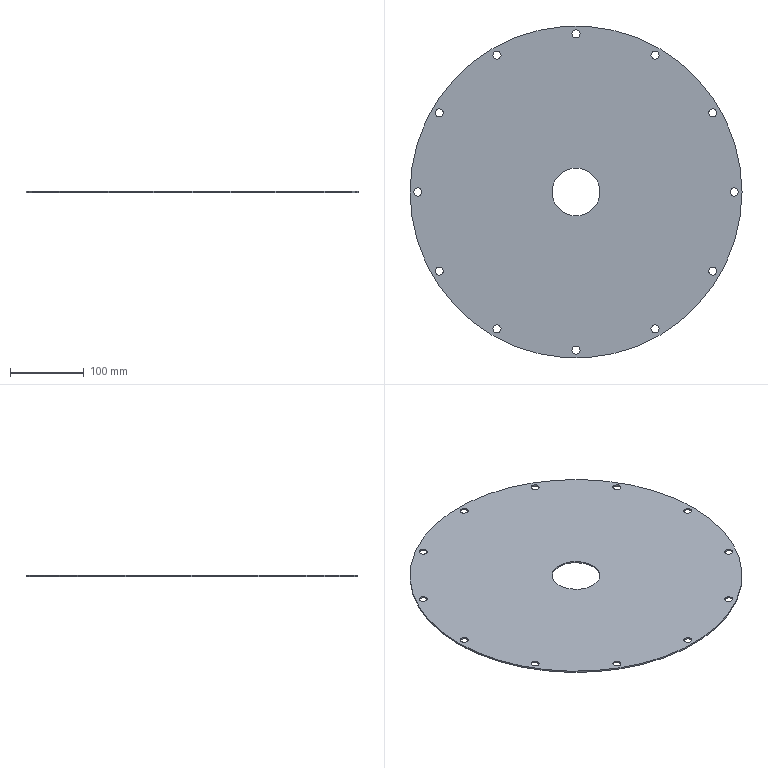Part | SolidWorks | features BaseBody 1 | 1 solid | 30 faces | box 450 x 450 x 2 mm | volume 309169 mm3 | cylinder 28 | plane 2 | commonest cylinder face diameters 11 x24 65 x2 450 x2
STEP:
#1=CARTESIAN_POINT('',(32.5,0.,2.));
#2=VERTEX_POINT('',#1);
#3=CARTESIAN_POINT('',(-32.5,0.,2.));
#4=VERTEX_POINT('',#3);
#5=CARTESIAN_POINT('',(0.,0.,2.));
#6=DIRECTION('',(0.,0.,-1.));
#7=DIRECTION('',(-1.,0.,0.));
#8=AXIS2_PLACEMENT_3D('',#5,#6,#7);
#9=CIRCLE('',#8,32.5);
#10=EDGE_CURVE('',#2,#4,#9,.T.);
#11=ORIENTED_EDGE('',*,*,#10,.F.);
#12=CARTESIAN_POINT('',(32.5,0.,0.));
#13=VERTEX_POINT('',#12);
#14=CARTESIAN_POINT('',(32.5,0.,2.));
#15=DIRECTION('',(0.,0.,-1.));
#16=VECTOR('',#15,1000.);
#17=LINE('',#14,#16);
#18=EDGE_CURVE('',#2,#13,#17,.T.);
#19=ORIENTED_EDGE('',*,*,#18,.T.);
#20=CARTESIAN_POINT('',(-32.5,0.,0.));
#21=VERTEX_POINT('',#20);
#22=CARTESIAN_POINT('',(0.,0.,0.));
#23=DIRECTION('',(0.,0.,1.));
#24=DIRECTION('',(-1.,0.,0.));
#25=AXIS2_PLACEMENT_3D('',#22,#23,#24);
#26=CIRCLE('',#25,32.5);
#27=EDGE_CURVE('',#21,#13,#26,.T.);
#28=ORIENTED_EDGE('',*,*,#27,.F.);
#29=CARTESIAN_POINT('',(-32.5,0.,2.));
#30=DIRECTION('',(0.,0.,-1.));
#31=VECTOR('',#30,1000.);
#32=LINE('',#29,#31);
#33=EDGE_CURVE('',#4,#21,#32,.T.);
#34=ORIENTED_EDGE('',*,*,#33,.F.);
#35=EDGE_LOOP('',(#11,#19,#28,#34));
#36=FACE_OUTER_BOUND('',#35,.T.);
#37=CARTESIAN_POINT('',(0.,0.,2.));
#38=DIRECTION('',(0.,0.,-1.));
#39=DIRECTION('',(-1.,0.,0.));
#40=AXIS2_PLACEMENT_3D('',#37,#38,#39);
#41=CYLINDRICAL_SURFACE('',#40,32.5);
#42=ADVANCED_FACE('',(#36),#41,.F.);
#43=CARTESIAN_POINT('',(-180.098,-107.155,2.));
#44=VERTEX_POINT('',#43);
#45=CARTESIAN_POINT('',(-191.098,-107.155,2.));
#46=VERTEX_POINT('',#45);
#47=CARTESIAN_POINT('',(-185.598,-107.155,2.));
#48=DIRECTION('',(0.,0.,-1.));
#49=DIRECTION('',(-1.,0.,0.));
#50=AXIS2_PLACEMENT_3D('',#47,#48,#49);
#51=CIRCLE('',#50,5.5);
#52=EDGE_CURVE('',#44,#46,#51,.T.);
#53=ORIENTED_EDGE('',*,*,#52,.F.);
#54=CARTESIAN_POINT('',(-180.098,-107.155,0.));
#55=VERTEX_POINT('',#54);
#56=CARTESIAN_POINT('',(-180.098,-107.155,2.));
#57=DIRECTION('',(0.,0.,-1.));
#58=VECTOR('',#57,1000.);
#59=LINE('',#56,#58);
#60=EDGE_CURVE('',#44,#55,#59,.T.);
#61=ORIENTED_EDGE('',*,*,#60,.T.);
#62=CARTESIAN_POINT('',(-191.098,-107.155,0.));
#63=VERTEX_POINT('',#62);
#64=CARTESIAN_POINT('',(-185.598,-107.155,0.));
#65=DIRECTION('',(0.,0.,1.));
#66=DIRECTION('',(-1.,0.,0.));
#67=AXIS2_PLACEMENT_3D('',#64,#65,#66);
#68=CIRCLE('',#67,5.5);
#69=EDGE_CURVE('',#63,#55,#68,.T.);
#70=ORIENTED_EDGE('',*,*,#69,.F.);
#71=CARTESIAN_POINT('',(-191.098,-107.155,2.));
#72=DIRECTION('',(0.,0.,-1.));
#73=VECTOR('',#72,1000.);
#74=LINE('',#71,#73);
#75=EDGE_CURVE('',#46,#63,#74,.T.);
#76=ORIENTED_EDGE('',*,*,#75,.F.);
#77=EDGE_LOOP('',(#53,#61,#70,#76));
#78=FACE_OUTER_BOUND('',#77,.T.);
#79=CARTESIAN_POINT('',(-185.598,-107.155,2.));
#80=DIRECTION('',(0.,0.,-1.));
#81=DIRECTION('',(-1.,0.,0.));
#82=AXIS2_PLACEMENT_3D('',#79,#80,#81);
#83=CYLINDRICAL_SURFACE('',#82,5.5);
#84=ADVANCED_FACE('',(#78),#83,.F.);
#85=CARTESIAN_POINT('',(5.5,-214.31,2.));
#86=VERTEX_POINT('',#85);
#87=CARTESIAN_POINT('',(-5.5,-214.31,2.));
#88=VERTEX_POINT('',#87);
#89=CARTESIAN_POINT('',(0.,-214.31,2.));
#90=DIRECTION('',(0.,0.,-1.));
#91=DIRECTION('',(-1.,0.,0.));
#92=AXIS2_PLACEMENT_3D('',#89,#90,#91);
#93=CIRCLE('',#92,5.5);
#94=EDGE_CURVE('',#86,#88,#93,.T.);
#95=ORIENTED_EDGE('',*,*,#94,.F.);
#96=CARTESIAN_POINT('',(5.5,-214.31,0.));
#97=VERTEX_POINT('',#96);
#98=CARTESIAN_POINT('',(5.5,-214.31,2.));
#99=DIRECTION('',(0.,0.,-1.));
#100=VECTOR('',#99,1000.);
#101=LINE('',#98,#100);
#102=EDGE_CURVE('',#86,#97,#101,.T.);
#103=ORIENTED_EDGE('',*,*,#102,.T.);
#104=CARTESIAN_POINT('',(-5.5,-214.31,0.));
#105=VERTEX_POINT('',#104);
#106=CARTESIAN_POINT('',(0.,-214.31,0.));
#107=DIRECTION('',(0.,0.,1.));
#108=DIRECTION('',(-1.,0.,0.));
#109=AXIS2_PLACEMENT_3D('',#106,#107,#108);
#110=CIRCLE('',#109,5.5);
#111=EDGE_CURVE('',#105,#97,#110,.T.);
#112=ORIENTED_EDGE('',*,*,#111,.F.);
#113=CARTESIAN_POINT('',(-5.5,-214.31,2.));
#114=DIRECTION('',(0.,0.,-1.));
#115=VECTOR('',#114,1000.);
#116=LINE('',#113,#115);
#117=EDGE_CURVE('',#88,#105,#116,.T.);
#118=ORIENTED_EDGE('',*,*,#117,.F.);
#119=EDGE_LOOP('',(#95,#103,#112,#118));
#120=FACE_OUTER_BOUND('',#119,.T.);
#121=CARTESIAN_POINT('',(0.,-214.31,2.));
#122=DIRECTION('',(0.,0.,-1.));
#123=DIRECTION('',(-1.,0.,0.));
#124=AXIS2_PLACEMENT_3D('',#121,#122,#123);
#125=CYLINDRICAL_SURFACE('',#124,5.5);
#126=ADVANCED_FACE('',(#120),#125,.F.);
#127=CARTESIAN_POINT('',(191.098,-107.155,2.));
#128=VERTEX_POINT('',#127);
#129=CARTESIAN_POINT('',(180.098,-107.155,2.));
#130=VERTEX_POINT('',#129);
#131=CARTESIAN_POINT('',(185.598,-107.155,2.));
#132=DIRECTION('',(0.,0.,-1.));
#133=DIRECTION('',(-1.,0.,0.));
#134=AXIS2_PLACEMENT_3D('',#131,#132,#133);
#135=CIRCLE('',#134,5.5);
#136=EDGE_CURVE('',#128,#130,#135,.T.);
#137=ORIENTED_EDGE('',*,*,#136,.F.);
#138=CARTESIAN_POINT('',(191.098,-107.155,0.));
#139=VERTEX_POINT('',#138);
#140=CARTESIAN_POINT('',(191.098,-107.155,2.));
#141=DIRECTION('',(0.,0.,-1.));
#142=VECTOR('',#141,1000.);
#143=LINE('',#140,#142);
#144=EDGE_CURVE('',#128,#139,#143,.T.);
#145=ORIENTED_EDGE('',*,*,#144,.T.);
#146=CARTESIAN_POINT('',(180.098,-107.155,0.));
#147=VERTEX_POINT('',#146);
#148=CARTESIAN_POINT('',(185.598,-107.155,0.));
#149=DIRECTION('',(0.,0.,1.));
#150=DIRECTION('',(-1.,0.,0.));
#151=AXIS2_PLACEMENT_3D('',#148,#149,#150);
#152=CIRCLE('',#151,5.5);
#153=EDGE_CURVE('',#147,#139,#152,.T.);
#154=ORIENTED_EDGE('',*,*,#153,.F.);
#155=CARTESIAN_POINT('',(180.098,-107.155,2.));
#156=DIRECTION('',(0.,0.,-1.));
#157=VECTOR('',#156,1000.);
#158=LINE('',#155,#157);
#159=EDGE_CURVE('',#130,#147,#158,.T.);
#160=ORIENTED_EDGE('',*,*,#159,.F.);
#161=EDGE_LOOP('',(#137,#145,#154,#160));
#162=FACE_OUTER_BOUND('',#161,.T.);
#163=CARTESIAN_POINT('',(185.598,-107.155,2.));
#164=DIRECTION('',(0.,0.,-1.));
#165=DIRECTION('',(-1.,0.,0.));
#166=AXIS2_PLACEMENT_3D('',#163,#164,#165);
#167=CYLINDRICAL_SURFACE('',#166,5.5);
#168=ADVANCED_FACE('',(#162),#167,.F.);
#169=CARTESIAN_POINT('',(191.098,107.155,2.));
#170=VERTEX_POINT('',#169);
#171=CARTESIAN_POINT('',(180.098,107.155,2.));
#172=VERTEX_POINT('',#171);
#173=CARTESIAN_POINT('',(185.598,107.155,2.));
#174=DIRECTION('',(0.,0.,-1.));
#175=DIRECTION('',(-1.,0.,0.));
#176=AXIS2_PLACEMENT_3D('',#173,#174,#175);
#177=CIRCLE('',#176,5.5);
#178=EDGE_CURVE('',#170,#172,#177,.T.);
#179=ORIENTED_EDGE('',*,*,#178,.F.);
#180=CARTESIAN_POINT('',(191.098,107.155,0.));
#181=VERTEX_POINT('',#180);
#182=CARTESIAN_POINT('',(191.098,107.155,2.));
#183=DIRECTION('',(0.,0.,-1.));
#184=VECTOR('',#183,1000.);
#185=LINE('',#182,#184);
#186=EDGE_CURVE('',#170,#181,#185,.T.);
#187=ORIENTED_EDGE('',*,*,#186,.T.);
#188=CARTESIAN_POINT('',(180.098,107.155,0.));
#189=VERTEX_POINT('',#188);
#190=CARTESIAN_POINT('',(185.598,107.155,0.));
#191=DIRECTION('',(0.,0.,1.));
#192=DIRECTION('',(-1.,0.,0.));
#193=AXIS2_PLACEMENT_3D('',#190,#191,#192);
#194=CIRCLE('',#193,5.5);
#195=EDGE_CURVE('',#189,#181,#194,.T.);
#196=ORIENTED_EDGE('',*,*,#195,.F.);
#197=CARTESIAN_POINT('',(180.098,107.155,2.));
#198=DIRECTION('',(0.,0.,-1.));
#199=VECTOR('',#198,1000.);
#200=LINE('',#197,#199);
#201=EDGE_CURVE('',#172,#189,#200,.T.);
#202=ORIENTED_EDGE('',*,*,#201,.F.);
#203=EDGE_LOOP('',(#179,#187,#196,#202));
#204=FACE_OUTER_BOUND('',#203,.T.);
#205=CARTESIAN_POINT('',(185.598,107.155,2.));
#206=DIRECTION('',(0.,0.,-1.));
#207=DIRECTION('',(-1.,0.,0.));
#208=AXIS2_PLACEMENT_3D('',#205,#206,#207);
#209=CYLINDRICAL_SURFACE('',#208,5.5);
#210=ADVANCED_FACE('',(#204),#209,.F.);
#211=CARTESIAN_POINT('',(5.5,214.31,2.));
#212=VERTEX_POINT('',#211);
#213=CARTESIAN_POINT('',(-5.5,214.31,2.));
#214=VERTEX_POINT('',#213);
#215=CARTESIAN_POINT('',(0.,214.31,2.));
#216=DIRECTION('',(0.,0.,-1.));
#217=DIRECTION('',(-1.,0.,0.));
#218=AXIS2_PLACEMENT_3D('',#215,#216,#217);
#219=CIRCLE('',#218,5.5);
#220=EDGE_CURVE('',#212,#214,#219,.T.);
#221=ORIENTED_EDGE('',*,*,#220,.F.);
#222=CARTESIAN_POINT('',(5.5,214.31,0.));
#223=VERTEX_POINT('',#222);
#224=CARTESIAN_POINT('',(5.5,214.31,2.));
#225=DIRECTION('',(0.,0.,-1.));
#226=VECTOR('',#225,1000.);
#227=LINE('',#224,#226);
#228=EDGE_CURVE('',#212,#223,#227,.T.);
#229=ORIENTED_EDGE('',*,*,#228,.T.);
#230=CARTESIAN_POINT('',(-5.5,214.31,0.));
#231=VERTEX_POINT('',#230);
#232=CARTESIAN_POINT('',(0.,214.31,0.));
#233=DIRECTION('',(0.,0.,1.));
#234=DIRECTION('',(-1.,0.,0.));
#235=AXIS2_PLACEMENT_3D('',#232,#233,#234);
#236=CIRCLE('',#235,5.5);
#237=EDGE_CURVE('',#231,#223,#236,.T.);
#238=ORIENTED_EDGE('',*,*,#237,.F.);
#239=CARTESIAN_POINT('',(-5.5,214.31,2.));
#240=DIRECTION('',(0.,0.,-1.));
#241=VECTOR('',#240,1000.);
#242=LINE('',#239,#241);
#243=EDGE_CURVE('',#214,#231,#242,.T.);
#244=ORIENTED_EDGE('',*,*,#243,.F.);
#245=EDGE_LOOP('',(#221,#229,#238,#244));
#246=FACE_OUTER_BOUND('',#245,.T.);
#247=CARTESIAN_POINT('',(0.,214.31,2.));
#248=DIRECTION('',(0.,0.,-1.));
#249=DIRECTION('',(-1.,0.,0.));
#250=AXIS2_PLACEMENT_3D('',#247,#248,#249);
#251=CYLINDRICAL_SURFACE('',#250,5.5);
#252=ADVANCED_FACE('',(#246),#251,.F.);
#253=CARTESIAN_POINT('',(-180.098,107.155,2.));
#254=VERTEX_POINT('',#253);
#255=CARTESIAN_POINT('',(-191.098,107.155,2.));
#256=VERTEX_POINT('',#255);
#257=CARTESIAN_POINT('',(-185.598,107.155,2.));
#258=DIRECTION('',(0.,0.,-1.));
#259=DIRECTION('',(-1.,0.,0.));
#260=AXIS2_PLACEMENT_3D('',#257,#258,#259);
#261=CIRCLE('',#260,5.5);
#262=EDGE_CURVE('',#254,#256,#261,.T.);
#263=ORIENTED_EDGE('',*,*,#262,.F.);
#264=CARTESIAN_POINT('',(-180.098,107.155,0.));
#265=VERTEX_POINT('',#264);
#266=CARTESIAN_POINT('',(-180.098,107.155,2.));
#267=DIRECTION('',(0.,0.,-1.));
#268=VECTOR('',#267,1000.);
#269=LINE('',#266,#268);
#270=EDGE_CURVE('',#254,#265,#269,.T.);
#271=ORIENTED_EDGE('',*,*,#270,.T.);
#272=CARTESIAN_POINT('',(-191.098,107.155,0.));
#273=VERTEX_POINT('',#272);
#274=CARTESIAN_POINT('',(-185.598,107.155,0.));
#275=DIRECTION('',(0.,0.,1.));
#276=DIRECTION('',(-1.,0.,0.));
#277=AXIS2_PLACEMENT_3D('',#274,#275,#276);
#278=CIRCLE('',#277,5.5);
#279=EDGE_CURVE('',#273,#265,#278,.T.);
#280=ORIENTED_EDGE('',*,*,#279,.F.);
#281=CARTESIAN_POINT('',(-191.098,107.155,2.));
#282=DIRECTION('',(0.,0.,-1.));
#283=VECTOR('',#282,1000.);
#284=LINE('',#281,#283);
#285=EDGE_CURVE('',#256,#273,#284,.T.);
#286=ORIENTED_EDGE('',*,*,#285,.F.);
#287=EDGE_LOOP('',(#263,#271,#280,#286));
#288=FACE_OUTER_BOUND('',#287,.T.);
#289=CARTESIAN_POINT('',(-185.598,107.155,2.));
#290=DIRECTION('',(0.,0.,-1.));
#291=DIRECTION('',(-1.,0.,0.));
#292=AXIS2_PLACEMENT_3D('',#289,#290,#291);
#293=CYLINDRICAL_SURFACE('',#292,5.5);
#294=ADVANCED_FACE('',(#288),#293,.F.);
#295=CARTESIAN_POINT('',(-101.655,185.598,2.));
#296=VERTEX_POINT('',#295);
#297=CARTESIAN_POINT('',(-112.655,185.598,2.));
#298=VERTEX_POINT('',#297);
#299=CARTESIAN_POINT('',(-107.155,185.598,2.));
#300=DIRECTION('',(0.,0.,-1.));
#301=DIRECTION('',(-1.,0.,0.));
#302=AXIS2_PLACEMENT_3D('',#299,#300,#301);
#303=CIRCLE('',#302,5.5);
#304=EDGE_CURVE('',#296,#298,#303,.T.);
#305=ORIENTED_EDGE('',*,*,#304,.F.);
#306=CARTESIAN_POINT('',(-101.655,185.598,0.));
#307=VERTEX_POINT('',#306);
#308=CARTESIAN_POINT('',(-101.655,185.598,2.));
#309=DIRECTION('',(0.,0.,-1.));
#310=VECTOR('',#309,1000.);
#311=LINE('',#308,#310);
#312=EDGE_CURVE('',#296,#307,#311,.T.);
#313=ORIENTED_EDGE('',*,*,#312,.T.);
#314=CARTESIAN_POINT('',(-112.655,185.598,0.));
#315=VERTEX_POINT('',#314);
#316=CARTESIAN_POINT('',(-107.155,185.598,0.));
#317=DIRECTION('',(0.,0.,1.));
#318=DIRECTION('',(-1.,0.,0.));
#319=AXIS2_PLACEMENT_3D('',#316,#317,#318);
#320=CIRCLE('',#319,5.5);
#321=EDGE_CURVE('',#315,#307,#320,.T.);
#322=ORIENTED_EDGE('',*,*,#321,.F.);
#323=CARTESIAN_POINT('',(-112.655,185.598,2.));
#324=DIRECTION('',(0.,0.,-1.));
#325=VECTOR('',#324,1000.);
#326=LINE('',#323,#325);
#327=EDGE_CURVE('',#298,#315,#326,.T.);
#328=ORIENTED_EDGE('',*,*,#327,.F.);
#329=EDGE_LOOP('',(#305,#313,#322,#328));
#330=FACE_OUTER_BOUND('',#329,.T.);
#331=CARTESIAN_POINT('',(-107.155,185.598,2.));
#332=DIRECTION('',(0.,0.,-1.));
#333=DIRECTION('',(-1.,0.,0.));
#334=AXIS2_PLACEMENT_3D('',#331,#332,#333);
#335=CYLINDRICAL_SURFACE('',#334,5.5);
#336=ADVANCED_FACE('',(#330),#335,.F.);
#337=CARTESIAN_POINT('',(112.655,185.598,2.));
#338=VERTEX_POINT('',#337);
#339=CARTESIAN_POINT('',(101.655,185.598,2.));
#340=VERTEX_POINT('',#339);
#341=CARTESIAN_POINT('',(107.155,185.598,2.));
#342=DIRECTION('',(0.,0.,-1.));
#343=DIRECTION('',(-1.,0.,0.));
#344=AXIS2_PLACEMENT_3D('',#341,#342,#343);
#345=CIRCLE('',#344,5.5);
#346=EDGE_CURVE('',#338,#340,#345,.T.);
#347=ORIENTED_EDGE('',*,*,#346,.F.);
#348=CARTESIAN_POINT('',(112.655,185.598,0.));
#349=VERTEX_POINT('',#348);
#350=CARTESIAN_POINT('',(112.655,185.598,2.));
#351=DIRECTION('',(0.,0.,-1.));
#352=VECTOR('',#351,1000.);
#353=LINE('',#350,#352);
#354=EDGE_CURVE('',#338,#349,#353,.T.);
#355=ORIENTED_EDGE('',*,*,#354,.T.);
#356=CARTESIAN_POINT('',(101.655,185.598,0.));
#357=VERTEX_POINT('',#356);
#358=CARTESIAN_POINT('',(107.155,185.598,0.));
#359=DIRECTION('',(0.,0.,1.));
#360=DIRECTION('',(-1.,0.,0.));
#361=AXIS2_PLACEMENT_3D('',#358,#359,#360);
#362=CIRCLE('',#361,5.5);
#363=EDGE_CURVE('',#357,#349,#362,.T.);
#364=ORIENTED_EDGE('',*,*,#363,.F.);
#365=CARTESIAN_POINT('',(101.655,185.598,2.));
#366=DIRECTION('',(0.,0.,-1.));
#367=VECTOR('',#366,1000.);
#368=LINE('',#365,#367);
#369=EDGE_CURVE('',#340,#357,#368,.T.);
#370=ORIENTED_EDGE('',*,*,#369,.F.);
#371=EDGE_LOOP('',(#347,#355,#364,#370));
#372=FACE_OUTER_BOUND('',#371,.T.);
#373=CARTESIAN_POINT('',(107.155,185.598,2.));
#374=DIRECTION('',(0.,0.,-1.));
#375=DIRECTION('',(-1.,0.,0.));
#376=AXIS2_PLACEMENT_3D('',#373,#374,#375);
#377=CYLINDRICAL_SURFACE('',#376,5.5);
#378=ADVANCED_FACE('',(#372),#377,.F.);
#379=CARTESIAN_POINT('',(219.81,0.,2.));
#380=VERTEX_POINT('',#379);
#381=CARTESIAN_POINT('',(208.81,0.,2.));
#382=VERTEX_POINT('',#381);
#383=CARTESIAN_POINT('',(214.31,0.,2.));
#384=DIRECTION('',(0.,0.,-1.));
#385=DIRECTION('',(-1.,0.,0.));
#386=AXIS2_PLACEMENT_3D('',#383,#384,#385);
#387=CIRCLE('',#386,5.5);
#388=EDGE_CURVE('',#380,#382,#387,.T.);
#389=ORIENTED_EDGE('',*,*,#388,.F.);
#390=CARTESIAN_POINT('',(219.81,0.,0.));
#391=VERTEX_POINT('',#390);
#392=CARTESIAN_POINT('',(219.81,0.,2.));
#393=DIRECTION('',(0.,0.,-1.));
#394=VECTOR('',#393,1000.);
#395=LINE('',#392,#394);
#396=EDGE_CURVE('',#380,#391,#395,.T.);
#397=ORIENTED_EDGE('',*,*,#396,.T.);
#398=CARTESIAN_POINT('',(208.81,0.,0.));
#399=VERTEX_POINT('',#398);
#400=CARTESIAN_POINT('',(214.31,0.,0.));
#401=DIRECTION('',(0.,0.,1.));
#402=DIRECTION('',(-1.,0.,0.));
#403=AXIS2_PLACEMENT_3D('',#400,#401,#402);
#404=CIRCLE('',#403,5.5);
#405=EDGE_CURVE('',#399,#391,#404,.T.);
#406=ORIENTED_EDGE('',*,*,#405,.F.);
#407=CARTESIAN_POINT('',(208.81,0.,2.));
#408=DIRECTION('',(0.,0.,-1.));
#409=VECTOR('',#408,1000.);
#410=LINE('',#407,#409);
#411=EDGE_CURVE('',#382,#399,#410,.T.);
#412=ORIENTED_EDGE('',*,*,#411,.F.);
#413=EDGE_LOOP('',(#389,#397,#406,#412));
#414=FACE_OUTER_BOUND('',#413,.T.);
#415=CARTESIAN_POINT('',(214.31,0.,2.));
#416=DIRECTION('',(0.,0.,-1.));
#417=DIRECTION('',(-1.,0.,0.));
#418=AXIS2_PLACEMENT_3D('',#415,#416,#417);
#419=CYLINDRICAL_SURFACE('',#418,5.5);
#420=ADVANCED_FACE('',(#414),#419,.F.);
#421=CARTESIAN_POINT('',(112.655,-185.598,2.));
#422=VERTEX_POINT('',#421);
#423=CARTESIAN_POINT('',(101.655,-185.598,2.));
#424=VERTEX_POINT('',#423);
#425=CARTESIAN_POINT('',(107.155,-185.598,2.));
#426=DIRECTION('',(0.,0.,-1.));
#427=DIRECTION('',(-1.,0.,0.));
#428=AXIS2_PLACEMENT_3D('',#425,#426,#427);
#429=CIRCLE('',#428,5.5);
#430=EDGE_CURVE('',#422,#424,#429,.T.);
#431=ORIENTED_EDGE('',*,*,#430,.F.);
#432=CARTESIAN_POINT('',(112.655,-185.598,0.));
#433=VERTEX_POINT('',#432);
#434=CARTESIAN_POINT('',(112.655,-185.598,2.));
#435=DIRECTION('',(0.,0.,-1.));
#436=VECTOR('',#435,1000.);
#437=LINE('',#434,#436);
#438=EDGE_CURVE('',#422,#433,#437,.T.);
#439=ORIENTED_EDGE('',*,*,#438,.T.);
#440=CARTESIAN_POINT('',(101.655,-185.598,0.));
#441=VERTEX_POINT('',#440);
#442=CARTESIAN_POINT('',(107.155,-185.598,0.));
#443=DIRECTION('',(0.,0.,1.));
#444=DIRECTION('',(-1.,0.,0.));
#445=AXIS2_PLACEMENT_3D('',#442,#443,#444);
#446=CIRCLE('',#445,5.5);
#447=EDGE_CURVE('',#441,#433,#446,.T.);
#448=ORIENTED_EDGE('',*,*,#447,.F.);
#449=CARTESIAN_POINT('',(101.655,-185.598,2.));
#450=DIRECTION('',(0.,0.,-1.));
#451=VECTOR('',#450,1000.);
#452=LINE('',#449,#451);
#453=EDGE_CURVE('',#424,#441,#452,.T.);
#454=ORIENTED_EDGE('',*,*,#453,.F.);
#455=EDGE_LOOP('',(#431,#439,#448,#454));
#456=FACE_OUTER_BOUND('',#455,.T.);
#457=CARTESIAN_POINT('',(107.155,-185.598,2.));
#458=DIRECTION('',(0.,0.,-1.));
#459=DIRECTION('',(-1.,0.,0.));
#460=AXIS2_PLACEMENT_3D('',#457,#458,#459);
#461=CYLINDRICAL_SURFACE('',#460,5.5);
#462=ADVANCED_FACE('',(#456),#461,.F.);
#463=CARTESIAN_POINT('',(-101.655,-185.598,2.));
#464=VERTEX_POINT('',#463);
#465=CARTESIAN_POINT('',(-112.655,-185.598,2.));
#466=VERTEX_POINT('',#465);
#467=CARTESIAN_POINT('',(-107.155,-185.598,2.));
#468=DIRECTION('',(0.,0.,-1.));
#469=DIRECTION('',(-1.,0.,0.));
#470=AXIS2_PLACEMENT_3D('',#467,#468,#469);
#471=CIRCLE('',#470,5.5);
#472=EDGE_CURVE('',#464,#466,#471,.T.);
#473=ORIENTED_EDGE('',*,*,#472,.F.);
#474=CARTESIAN_POINT('',(-101.655,-185.598,0.));
#475=VERTEX_POINT('',#474);
#476=CARTESIAN_POINT('',(-101.655,-185.598,2.));
#477=DIRECTION('',(0.,0.,-1.));
#478=VECTOR('',#477,1000.);
#479=LINE('',#476,#478);
#480=EDGE_CURVE('',#464,#475,#479,.T.);
#481=ORIENTED_EDGE('',*,*,#480,.T.);
#482=CARTESIAN_POINT('',(-112.655,-185.598,0.));
#483=VERTEX_POINT('',#482);
#484=CARTESIAN_POINT('',(-107.155,-185.598,0.));
#485=DIRECTION('',(0.,0.,1.));
#486=DIRECTION('',(-1.,0.,0.));
#487=AXIS2_PLACEMENT_3D('',#484,#485,#486);
#488=CIRCLE('',#487,5.5);
#489=EDGE_CURVE('',#483,#475,#488,.T.);
#490=ORIENTED_EDGE('',*,*,#489,.F.);
#491=CARTESIAN_POINT('',(-112.655,-185.598,2.));
#492=DIRECTION('',(0.,0.,-1.));
#493=VECTOR('',#492,1000.);
#494=LINE('',#491,#493);
#495=EDGE_CURVE('',#466,#483,#494,.T.);
#496=ORIENTED_EDGE('',*,*,#495,.F.);
#497=EDGE_LOOP('',(#473,#481,#490,#496));
#498=FACE_OUTER_BOUND('',#497,.T.);
#499=CARTESIAN_POINT('',(-107.155,-185.598,2.));
#500=DIRECTION('',(0.,0.,-1.));
#501=DIRECTION('',(-1.,0.,0.));
#502=AXIS2_PLACEMENT_3D('',#499,#500,#501);
#503=CYLINDRICAL_SURFACE('',#502,5.5);
#504=ADVANCED_FACE('',(#498),#503,.F.);
#505=CARTESIAN_POINT('',(-208.81,0.,2.));
#506=VERTEX_POINT('',#505);
#507=CARTESIAN_POINT('',(-219.81,0.,2.));
#508=VERTEX_POINT('',#507);
#509=CARTESIAN_POINT('',(-214.31,0.,2.));
#510=DIRECTION('',(0.,0.,-1.));
#511=DIRECTION('',(-1.,0.,0.));
#512=AXIS2_PLACEMENT_3D('',#509,#510,#511);
#513=CIRCLE('',#512,5.5);
#514=EDGE_CURVE('',#506,#508,#513,.T.);
#515=ORIENTED_EDGE('',*,*,#514,.F.);
#516=CARTESIAN_POINT('',(-208.81,0.,0.));
#517=VERTEX_POINT('',#516);
#518=CARTESIAN_POINT('',(-208.81,0.,2.));
#519=DIRECTION('',(0.,0.,-1.));
#520=VECTOR('',#519,1000.);
#521=LINE('',#518,#520);
#522=EDGE_CURVE('',#506,#517,#521,.T.);
#523=ORIENTED_EDGE('',*,*,#522,.T.);
#524=CARTESIAN_POINT('',(-219.81,0.,0.));
#525=VERTEX_POINT('',#524);
#526=CARTESIAN_POINT('',(-214.31,0.,0.));
#527=DIRECTION('',(0.,0.,1.));
#528=DIRECTION('',(-1.,0.,0.));
#529=AXIS2_PLACEMENT_3D('',#526,#527,#528);
#530=CIRCLE('',#529,5.5);
#531=EDGE_CURVE('',#525,#517,#530,.T.);
#532=ORIENTED_EDGE('',*,*,#531,.F.);
#533=CARTESIAN_POINT('',(-219.81,0.,2.));
#534=DIRECTION('',(0.,0.,-1.));
#535=VECTOR('',#534,1000.);
#536=LINE('',#533,#535);
#537=EDGE_CURVE('',#508,#525,#536,.T.);
#538=ORIENTED_EDGE('',*,*,#537,.F.);
#539=EDGE_LOOP('',(#515,#523,#532,#538));
#540=FACE_OUTER_BOUND('',#539,.T.);
#541=CARTESIAN_POINT('',(-214.31,0.,2.));
#542=DIRECTION('',(0.,0.,-1.));
#543=DIRECTION('',(-1.,0.,0.));
#544=AXIS2_PLACEMENT_3D('',#541,#542,#543);
#545=CYLINDRICAL_SURFACE('',#544,5.5);
#546=ADVANCED_FACE('',(#540),#545,.F.);
#547=CARTESIAN_POINT('',(225.,0.,2.));
#548=VERTEX_POINT('',#547);
#549=CARTESIAN_POINT('',(-225.,0.,2.));
#550=VERTEX_POINT('',#549);
#551=CARTESIAN_POINT('',(0.,0.,2.));
#552=DIRECTION('',(0.,0.,1.));
#553=DIRECTION('',(-1.,0.,0.));
#554=AXIS2_PLACEMENT_3D('',#551,#552,#553);
#555=CIRCLE('',#554,225.);
#556=EDGE_CURVE('',#548,#550,#555,.T.);
#557=ORIENTED_EDGE('',*,*,#556,.F.);
#558=CARTESIAN_POINT('',(225.,0.,0.));
#559=VERTEX_POINT('',#558);
#560=CARTESIAN_POINT('',(225.,0.,2.));
#561=DIRECTION('',(0.,0.,-1.));
#562=VECTOR('',#561,1000.);
#563=LINE('',#560,#562);
#564=EDGE_CURVE('',#548,#559,#563,.T.);
#565=ORIENTED_EDGE('',*,*,#564,.T.);
#566=CARTESIAN_POINT('',(-225.,0.,0.));
#567=VERTEX_POINT('',#566);
#568=CARTESIAN_POINT('',(0.,0.,0.));
#569=DIRECTION('',(0.,0.,1.));
#570=DIRECTION('',(-1.,0.,0.));
#571=AXIS2_PLACEMENT_3D('',#568,#569,#570);
#572=CIRCLE('',#571,225.);
#573=EDGE_CURVE('',#559,#567,#572,.T.);
#574=ORIENTED_EDGE('',*,*,#573,.T.);
#575=CARTESIAN_POINT('',(-225.,0.,2.));
#576=DIRECTION('',(0.,0.,-1.));
#577=VECTOR('',#576,1000.);
#578=LINE('',#575,#577);
#579=EDGE_CURVE('',#550,#567,#578,.T.);
#580=ORIENTED_EDGE('',*,*,#579,.F.);
#581=EDGE_LOOP('',(#557,#565,#574,#580));
#582=FACE_OUTER_BOUND('',#581,.T.);
#583=CARTESIAN_POINT('',(0.,0.,2.));
#584=DIRECTION('',(0.,0.,-1.));
#585=DIRECTION('',(-1.,0.,0.));
#586=AXIS2_PLACEMENT_3D('',#583,#584,#585);
#587=CYLINDRICAL_SURFACE('',#586,225.);
#588=ADVANCED_FACE('',(#582),#587,.T.);
#589=CARTESIAN_POINT('',(0.,0.,2.));
#590=DIRECTION('',(0.,0.,-1.));
#591=DIRECTION('',(-1.,0.,0.));
#592=AXIS2_PLACEMENT_3D('',#589,#590,#591);
#593=CIRCLE('',#592,32.5);
#594=EDGE_CURVE('',#4,#2,#593,.T.);
#595=ORIENTED_EDGE('',*,*,#594,.T.);
#596=ORIENTED_EDGE('',*,*,#10,.T.);
#597=EDGE_LOOP('',(#595,#596));
#598=FACE_BOUND('',#597,.T.);
#599=CARTESIAN_POINT('',(-185.598,-107.155,2.));
#600=DIRECTION('',(0.,0.,-1.));
#601=DIRECTION('',(-1.,0.,0.));
#602=AXIS2_PLACEMENT_3D('',#599,#600,#601);
#603=CIRCLE('',#602,5.5);
#604=EDGE_CURVE('',#46,#44,#603,.T.);
#605=ORIENTED_EDGE('',*,*,#604,.T.);
#606=ORIENTED_EDGE('',*,*,#52,.T.);
#607=EDGE_LOOP('',(#605,#606));
#608=FACE_BOUND('',#607,.T.);
#609=CARTESIAN_POINT('',(0.,-214.31,2.));
#610=DIRECTION('',(0.,0.,-1.));
#611=DIRECTION('',(-1.,0.,0.));
#612=AXIS2_PLACEMENT_3D('',#609,#610,#611);
#613=CIRCLE('',#612,5.5);
#614=EDGE_CURVE('',#88,#86,#613,.T.);
#615=ORIENTED_EDGE('',*,*,#614,.T.);
#616=ORIENTED_EDGE('',*,*,#94,.T.);
#617=EDGE_LOOP('',(#615,#616));
#618=FACE_BOUND('',#617,.T.);
#619=CARTESIAN_POINT('',(185.598,-107.155,2.));
#620=DIRECTION('',(0.,0.,-1.));
#621=DIRECTION('',(-1.,0.,0.));
#622=AXIS2_PLACEMENT_3D('',#619,#620,#621);
#623=CIRCLE('',#622,5.5);
#624=EDGE_CURVE('',#130,#128,#623,.T.);
#625=ORIENTED_EDGE('',*,*,#624,.T.);
#626=ORIENTED_EDGE('',*,*,#136,.T.);
#627=EDGE_LOOP('',(#625,#626));
#628=FACE_BOUND('',#627,.T.);
#629=CARTESIAN_POINT('',(185.598,107.155,2.));
#630=DIRECTION('',(0.,0.,-1.));
#631=DIRECTION('',(-1.,0.,0.));
#632=AXIS2_PLACEMENT_3D('',#629,#630,#631);
#633=CIRCLE('',#632,5.5);
#634=EDGE_CURVE('',#172,#170,#633,.T.);
#635=ORIENTED_EDGE('',*,*,#634,.T.);
#636=ORIENTED_EDGE('',*,*,#178,.T.);
#637=EDGE_LOOP('',(#635,#636));
#638=FACE_BOUND('',#637,.T.);
#639=CARTESIAN_POINT('',(0.,214.31,2.));
#640=DIRECTION('',(0.,0.,-1.));
#641=DIRECTION('',(-1.,0.,0.));
#642=AXIS2_PLACEMENT_3D('',#639,#640,#641);
#643=CIRCLE('',#642,5.5);
#644=EDGE_CURVE('',#214,#212,#643,.T.);
#645=ORIENTED_EDGE('',*,*,#644,.T.);
#646=ORIENTED_EDGE('',*,*,#220,.T.);
#647=EDGE_LOOP('',(#645,#646));
#648=FACE_BOUND('',#647,.T.);
#649=CARTESIAN_POINT('',(-185.598,107.155,2.));
#650=DIRECTION('',(0.,0.,-1.));
#651=DIRECTION('',(-1.,0.,0.));
#652=AXIS2_PLACEMENT_3D('',#649,#650,#651);
#653=CIRCLE('',#652,5.5);
#654=EDGE_CURVE('',#256,#254,#653,.T.);
#655=ORIENTED_EDGE('',*,*,#654,.T.);
#656=ORIENTED_EDGE('',*,*,#262,.T.);
#657=EDGE_LOOP('',(#655,#656));
#658=FACE_BOUND('',#657,.T.);
#659=CARTESIAN_POINT('',(-107.155,185.598,2.));
#660=DIRECTION('',(0.,0.,-1.));
#661=DIRECTION('',(-1.,0.,0.));
#662=AXIS2_PLACEMENT_3D('',#659,#660,#661);
#663=CIRCLE('',#662,5.5);
#664=EDGE_CURVE('',#298,#296,#663,.T.);
#665=ORIENTED_EDGE('',*,*,#664,.T.);
#666=ORIENTED_EDGE('',*,*,#304,.T.);
#667=EDGE_LOOP('',(#665,#666));
#668=FACE_BOUND('',#667,.T.);
#669=CARTESIAN_POINT('',(107.155,185.598,2.));
#670=DIRECTION('',(0.,0.,-1.));
#671=DIRECTION('',(-1.,0.,0.));
#672=AXIS2_PLACEMENT_3D('',#669,#670,#671);
#673=CIRCLE('',#672,5.5);
#674=EDGE_CURVE('',#340,#338,#673,.T.);
#675=ORIENTED_EDGE('',*,*,#674,.T.);
#676=ORIENTED_EDGE('',*,*,#346,.T.);
#677=EDGE_LOOP('',(#675,#676));
#678=FACE_BOUND('',#677,.T.);
#679=CARTESIAN_POINT('',(214.31,0.,2.));
#680=DIRECTION('',(0.,0.,-1.));
#681=DIRECTION('',(-1.,0.,0.));
#682=AXIS2_PLACEMENT_3D('',#679,#680,#681);
#683=CIRCLE('',#682,5.5);
#684=EDGE_CURVE('',#382,#380,#683,.T.);
#685=ORIENTED_EDGE('',*,*,#684,.T.);
#686=ORIENTED_EDGE('',*,*,#388,.T.);
#687=EDGE_LOOP('',(#685,#686));
#688=FACE_BOUND('',#687,.T.);
#689=CARTESIAN_POINT('',(107.155,-185.598,2.));
#690=DIRECTION('',(0.,0.,-1.));
#691=DIRECTION('',(-1.,0.,0.));
#692=AXIS2_PLACEMENT_3D('',#689,#690,#691);
#693=CIRCLE('',#692,5.5);
#694=EDGE_CURVE('',#424,#422,#693,.T.);
#695=ORIENTED_EDGE('',*,*,#694,.T.);
#696=ORIENTED_EDGE('',*,*,#430,.T.);
#697=EDGE_LOOP('',(#695,#696));
#698=FACE_BOUND('',#697,.T.);
#699=CARTESIAN_POINT('',(-107.155,-185.598,2.));
#700=DIRECTION('',(0.,0.,-1.));
#701=DIRECTION('',(-1.,0.,0.));
#702=AXIS2_PLACEMENT_3D('',#699,#700,#701);
#703=CIRCLE('',#702,5.5);
#704=EDGE_CURVE('',#466,#464,#703,.T.);
#705=ORIENTED_EDGE('',*,*,#704,.T.);
#706=ORIENTED_EDGE('',*,*,#472,.T.);
#707=EDGE_LOOP('',(#705,#706));
#708=FACE_BOUND('',#707,.T.);
#709=CARTESIAN_POINT('',(-214.31,0.,2.));
#710=DIRECTION('',(0.,0.,-1.));
#711=DIRECTION('',(-1.,0.,0.));
#712=AXIS2_PLACEMENT_3D('',#709,#710,#711);
#713=CIRCLE('',#712,5.5);
#714=EDGE_CURVE('',#508,#506,#713,.T.);
#715=ORIENTED_EDGE('',*,*,#714,.T.);
#716=ORIENTED_EDGE('',*,*,#514,.T.);
#717=EDGE_LOOP('',(#715,#716));
#718=FACE_BOUND('',#717,.T.);
#719=CARTESIAN_POINT('',(0.,0.,2.));
#720=DIRECTION('',(0.,0.,1.));
#721=DIRECTION('',(-1.,0.,0.));
#722=AXIS2_PLACEMENT_3D('',#719,#720,#721);
#723=CIRCLE('',#722,225.);
#724=EDGE_CURVE('',#550,#548,#723,.T.);
#725=ORIENTED_EDGE('',*,*,#724,.T.);
#726=ORIENTED_EDGE('',*,*,#556,.T.);
#727=EDGE_LOOP('',(#725,#726));
#728=FACE_OUTER_BOUND('',#727,.T.);
#729=CARTESIAN_POINT('',(0.,0.,2.));
#730=DIRECTION('',(0.,0.,1.));
#731=DIRECTION('',(1.,0.,0.));
#732=AXIS2_PLACEMENT_3D('',#729,#730,#731);
#733=PLANE('',#732);
#734=ADVANCED_FACE('',(#598,#608,#618,#628,#638,#648,#658,#668,#678,#688,#698,#708,#718,#728),#733,.T.);
#735=ORIENTED_EDGE('',*,*,#18,.F.);
#736=ORIENTED_EDGE('',*,*,#594,.F.);
#737=ORIENTED_EDGE('',*,*,#33,.T.);
#738=CARTESIAN_POINT('',(0.,0.,0.));
#739=DIRECTION('',(0.,0.,1.));
#740=DIRECTION('',(-1.,0.,0.));
#741=AXIS2_PLACEMENT_3D('',#738,#739,#740);
#742=CIRCLE('',#741,32.5);
#743=EDGE_CURVE('',#13,#21,#742,.T.);
#744=ORIENTED_EDGE('',*,*,#743,.F.);
#745=EDGE_LOOP('',(#735,#736,#737,#744));
#746=FACE_OUTER_BOUND('',#745,.T.);
#747=CARTESIAN_POINT('',(0.,0.,2.));
#748=DIRECTION('',(0.,0.,-1.));
#749=DIRECTION('',(-1.,0.,0.));
#750=AXIS2_PLACEMENT_3D('',#747,#748,#749);
#751=CYLINDRICAL_SURFACE('',#750,32.5);
#752=ADVANCED_FACE('',(#746),#751,.F.);
#753=ORIENTED_EDGE('',*,*,#60,.F.);
#754=ORIENTED_EDGE('',*,*,#604,.F.);
#755=ORIENTED_EDGE('',*,*,#75,.T.);
#756=CARTESIAN_POINT('',(-185.598,-107.155,0.));
#757=DIRECTION('',(0.,0.,1.));
#758=DIRECTION('',(-1.,0.,0.));
#759=AXIS2_PLACEMENT_3D('',#756,#757,#758);
#760=CIRCLE('',#759,5.5);
#761=EDGE_CURVE('',#55,#63,#760,.T.);
#762=ORIENTED_EDGE('',*,*,#761,.F.);
#763=EDGE_LOOP('',(#753,#754,#755,#762));
#764=FACE_OUTER_BOUND('',#763,.T.);
#765=CARTESIAN_POINT('',(-185.598,-107.155,2.));
#766=DIRECTION('',(0.,0.,-1.));
#767=DIRECTION('',(-1.,0.,0.));
#768=AXIS2_PLACEMENT_3D('',#765,#766,#767);
#769=CYLINDRICAL_SURFACE('',#768,5.5);
#770=ADVANCED_FACE('',(#764),#769,.F.);
#771=ORIENTED_EDGE('',*,*,#102,.F.);
#772=ORIENTED_EDGE('',*,*,#614,.F.);
#773=ORIENTED_EDGE('',*,*,#117,.T.);
#774=CARTESIAN_POINT('',(0.,-214.31,0.));
#775=DIRECTION('',(0.,0.,1.));
#776=DIRECTION('',(-1.,0.,0.));
#777=AXIS2_PLACEMENT_3D('',#774,#775,#776);
#778=CIRCLE('',#777,5.5);
#779=EDGE_CURVE('',#97,#105,#778,.T.);
#780=ORIENTED_EDGE('',*,*,#779,.F.);
#781=EDGE_LOOP('',(#771,#772,#773,#780));
#782=FACE_OUTER_BOUND('',#781,.T.);
#783=CARTESIAN_POINT('',(0.,-214.31,2.));
#784=DIRECTION('',(0.,0.,-1.));
#785=DIRECTION('',(-1.,0.,0.));
#786=AXIS2_PLACEMENT_3D('',#783,#784,#785);
#787=CYLINDRICAL_SURFACE('',#786,5.5);
#788=ADVANCED_FACE('',(#782),#787,.F.);
#789=ORIENTED_EDGE('',*,*,#144,.F.);
#790=ORIENTED_EDGE('',*,*,#624,.F.);
#791=ORIENTED_EDGE('',*,*,#159,.T.);
#792=CARTESIAN_POINT('',(185.598,-107.155,0.));
#793=DIRECTION('',(0.,0.,1.));
#794=DIRECTION('',(-1.,0.,0.));
#795=AXIS2_PLACEMENT_3D('',#792,#793,#794);
#796=CIRCLE('',#795,5.5);
#797=EDGE_CURVE('',#139,#147,#796,.T.);
#798=ORIENTED_EDGE('',*,*,#797,.F.);
#799=EDGE_LOOP('',(#789,#790,#791,#798));
#800=FACE_OUTER_BOUND('',#799,.T.);
#801=CARTESIAN_POINT('',(185.598,-107.155,2.));
#802=DIRECTION('',(0.,0.,-1.));
#803=DIRECTION('',(-1.,0.,0.));
#804=AXIS2_PLACEMENT_3D('',#801,#802,#803);
#805=CYLINDRICAL_SURFACE('',#804,5.5);
#806=ADVANCED_FACE('',(#800),#805,.F.);
#807=ORIENTED_EDGE('',*,*,#186,.F.);
#808=ORIENTED_EDGE('',*,*,#634,.F.);
#809=ORIENTED_EDGE('',*,*,#201,.T.);
#810=CARTESIAN_POINT('',(185.598,107.155,0.));
#811=DIRECTION('',(0.,0.,1.));
#812=DIRECTION('',(-1.,0.,0.));
#813=AXIS2_PLACEMENT_3D('',#810,#811,#812);
#814=CIRCLE('',#813,5.5);
#815=EDGE_CURVE('',#181,#189,#814,.T.);
#816=ORIENTED_EDGE('',*,*,#815,.F.);
#817=EDGE_LOOP('',(#807,#808,#809,#816));
#818=FACE_OUTER_BOUND('',#817,.T.);
#819=CARTESIAN_POINT('',(185.598,107.155,2.));
#820=DIRECTION('',(0.,0.,-1.));
#821=DIRECTION('',(-1.,0.,0.));
#822=AXIS2_PLACEMENT_3D('',#819,#820,#821);
#823=CYLINDRICAL_SURFACE('',#822,5.5);
#824=ADVANCED_FACE('',(#818),#823,.F.);
#825=ORIENTED_EDGE('',*,*,#228,.F.);
#826=ORIENTED_EDGE('',*,*,#644,.F.);
#827=ORIENTED_EDGE('',*,*,#243,.T.);
#828=CARTESIAN_POINT('',(0.,214.31,0.));
#829=DIRECTION('',(0.,0.,1.));
#830=DIRECTION('',(-1.,0.,0.));
#831=AXIS2_PLACEMENT_3D('',#828,#829,#830);
#832=CIRCLE('',#831,5.5);
#833=EDGE_CURVE('',#223,#231,#832,.T.);
#834=ORIENTED_EDGE('',*,*,#833,.F.);
#835=EDGE_LOOP('',(#825,#826,#827,#834));
#836=FACE_OUTER_BOUND('',#835,.T.);
#837=CARTESIAN_POINT('',(0.,214.31,2.));
#838=DIRECTION('',(0.,0.,-1.));
#839=DIRECTION('',(-1.,0.,0.));
#840=AXIS2_PLACEMENT_3D('',#837,#838,#839);
#841=CYLINDRICAL_SURFACE('',#840,5.5);
#842=ADVANCED_FACE('',(#836),#841,.F.);
#843=ORIENTED_EDGE('',*,*,#270,.F.);
#844=ORIENTED_EDGE('',*,*,#654,.F.);
#845=ORIENTED_EDGE('',*,*,#285,.T.);
#846=CARTESIAN_POINT('',(-185.598,107.155,0.));
#847=DIRECTION('',(0.,0.,1.));
#848=DIRECTION('',(-1.,0.,0.));
#849=AXIS2_PLACEMENT_3D('',#846,#847,#848);
#850=CIRCLE('',#849,5.5);
#851=EDGE_CURVE('',#265,#273,#850,.T.);
#852=ORIENTED_EDGE('',*,*,#851,.F.);
#853=EDGE_LOOP('',(#843,#844,#845,#852));
#854=FACE_OUTER_BOUND('',#853,.T.);
#855=CARTESIAN_POINT('',(-185.598,107.155,2.));
#856=DIRECTION('',(0.,0.,-1.));
#857=DIRECTION('',(-1.,0.,0.));
#858=AXIS2_PLACEMENT_3D('',#855,#856,#857);
#859=CYLINDRICAL_SURFACE('',#858,5.5);
#860=ADVANCED_FACE('',(#854),#859,.F.);
#861=ORIENTED_EDGE('',*,*,#312,.F.);
#862=ORIENTED_EDGE('',*,*,#664,.F.);
#863=ORIENTED_EDGE('',*,*,#327,.T.);
#864=CARTESIAN_POINT('',(-107.155,185.598,0.));
#865=DIRECTION('',(0.,0.,1.));
#866=DIRECTION('',(-1.,0.,0.));
#867=AXIS2_PLACEMENT_3D('',#864,#865,#866);
#868=CIRCLE('',#867,5.5);
#869=EDGE_CURVE('',#307,#315,#868,.T.);
#870=ORIENTED_EDGE('',*,*,#869,.F.);
#871=EDGE_LOOP('',(#861,#862,#863,#870));
#872=FACE_OUTER_BOUND('',#871,.T.);
#873=CARTESIAN_POINT('',(-107.155,185.598,2.));
#874=DIRECTION('',(0.,0.,-1.));
#875=DIRECTION('',(-1.,0.,0.));
#876=AXIS2_PLACEMENT_3D('',#873,#874,#875);
#877=CYLINDRICAL_SURFACE('',#876,5.5);
#878=ADVANCED_FACE('',(#872),#877,.F.);
#879=ORIENTED_EDGE('',*,*,#354,.F.);
#880=ORIENTED_EDGE('',*,*,#674,.F.);
#881=ORIENTED_EDGE('',*,*,#369,.T.);
#882=CARTESIAN_POINT('',(107.155,185.598,0.));
#883=DIRECTION('',(0.,0.,1.));
#884=DIRECTION('',(-1.,0.,0.));
#885=AXIS2_PLACEMENT_3D('',#882,#883,#884);
#886=CIRCLE('',#885,5.5);
#887=EDGE_CURVE('',#349,#357,#886,.T.);
#888=ORIENTED_EDGE('',*,*,#887,.F.);
#889=EDGE_LOOP('',(#879,#880,#881,#888));
#890=FACE_OUTER_BOUND('',#889,.T.);
#891=CARTESIAN_POINT('',(107.155,185.598,2.));
#892=DIRECTION('',(0.,0.,-1.));
#893=DIRECTION('',(-1.,0.,0.));
#894=AXIS2_PLACEMENT_3D('',#891,#892,#893);
#895=CYLINDRICAL_SURFACE('',#894,5.5);
#896=ADVANCED_FACE('',(#890),#895,.F.);
#897=ORIENTED_EDGE('',*,*,#396,.F.);
#898=ORIENTED_EDGE('',*,*,#684,.F.);
#899=ORIENTED_EDGE('',*,*,#411,.T.);
#900=CARTESIAN_POINT('',(214.31,0.,0.));
#901=DIRECTION('',(0.,0.,1.));
#902=DIRECTION('',(-1.,0.,0.));
#903=AXIS2_PLACEMENT_3D('',#900,#901,#902);
#904=CIRCLE('',#903,5.5);
#905=EDGE_CURVE('',#391,#399,#904,.T.);
#906=ORIENTED_EDGE('',*,*,#905,.F.);
#907=EDGE_LOOP('',(#897,#898,#899,#906));
#908=FACE_OUTER_BOUND('',#907,.T.);
#909=CARTESIAN_POINT('',(214.31,0.,2.));
#910=DIRECTION('',(0.,0.,-1.));
#911=DIRECTION('',(-1.,0.,0.));
#912=AXIS2_PLACEMENT_3D('',#909,#910,#911);
#913=CYLINDRICAL_SURFACE('',#912,5.5);
#914=ADVANCED_FACE('',(#908),#913,.F.);
#915=ORIENTED_EDGE('',*,*,#438,.F.);
#916=ORIENTED_EDGE('',*,*,#694,.F.);
#917=ORIENTED_EDGE('',*,*,#453,.T.);
#918=CARTESIAN_POINT('',(107.155,-185.598,0.));
#919=DIRECTION('',(0.,0.,1.));
#920=DIRECTION('',(-1.,0.,0.));
#921=AXIS2_PLACEMENT_3D('',#918,#919,#920);
#922=CIRCLE('',#921,5.5);
#923=EDGE_CURVE('',#433,#441,#922,.T.);
#924=ORIENTED_EDGE('',*,*,#923,.F.);
#925=EDGE_LOOP('',(#915,#916,#917,#924));
#926=FACE_OUTER_BOUND('',#925,.T.);
#927=CARTESIAN_POINT('',(107.155,-185.598,2.));
#928=DIRECTION('',(0.,0.,-1.));
#929=DIRECTION('',(-1.,0.,0.));
#930=AXIS2_PLACEMENT_3D('',#927,#928,#929);
#931=CYLINDRICAL_SURFACE('',#930,5.5);
#932=ADVANCED_FACE('',(#926),#931,.F.);
#933=ORIENTED_EDGE('',*,*,#480,.F.);
#934=ORIENTED_EDGE('',*,*,#704,.F.);
#935=ORIENTED_EDGE('',*,*,#495,.T.);
#936=CARTESIAN_POINT('',(-107.155,-185.598,0.));
#937=DIRECTION('',(0.,0.,1.));
#938=DIRECTION('',(-1.,0.,0.));
#939=AXIS2_PLACEMENT_3D('',#936,#937,#938);
#940=CIRCLE('',#939,5.5);
#941=EDGE_CURVE('',#475,#483,#940,.T.);
#942=ORIENTED_EDGE('',*,*,#941,.F.);
#943=EDGE_LOOP('',(#933,#934,#935,#942));
#944=FACE_OUTER_BOUND('',#943,.T.);
#945=CARTESIAN_POINT('',(-107.155,-185.598,2.));
#946=DIRECTION('',(0.,0.,-1.));
#947=DIRECTION('',(-1.,0.,0.));
#948=AXIS2_PLACEMENT_3D('',#945,#946,#947);
#949=CYLINDRICAL_SURFACE('',#948,5.5);
#950=ADVANCED_FACE('',(#944),#949,.F.);
#951=ORIENTED_EDGE('',*,*,#522,.F.);
#952=ORIENTED_EDGE('',*,*,#714,.F.);
#953=ORIENTED_EDGE('',*,*,#537,.T.);
#954=CARTESIAN_POINT('',(-214.31,0.,0.));
#955=DIRECTION('',(0.,0.,1.));
#956=DIRECTION('',(-1.,0.,0.));
#957=AXIS2_PLACEMENT_3D('',#954,#955,#956);
#958=CIRCLE('',#957,5.5);
#959=EDGE_CURVE('',#517,#525,#958,.T.);
#960=ORIENTED_EDGE('',*,*,#959,.F.);
#961=EDGE_LOOP('',(#951,#952,#953,#960));
#962=FACE_OUTER_BOUND('',#961,.T.);
#963=CARTESIAN_POINT('',(-214.31,0.,2.));
#964=DIRECTION('',(0.,0.,-1.));
#965=DIRECTION('',(-1.,0.,0.));
#966=AXIS2_PLACEMENT_3D('',#963,#964,#965);
#967=CYLINDRICAL_SURFACE('',#966,5.5);
#968=ADVANCED_FACE('',(#962),#967,.F.);
#969=ORIENTED_EDGE('',*,*,#564,.F.);
#970=ORIENTED_EDGE('',*,*,#724,.F.);
#971=ORIENTED_EDGE('',*,*,#579,.T.);
#972=CARTESIAN_POINT('',(0.,0.,0.));
#973=DIRECTION('',(0.,0.,1.));
#974=DIRECTION('',(-1.,0.,0.));
#975=AXIS2_PLACEMENT_3D('',#972,#973,#974);
#976=CIRCLE('',#975,225.);
#977=EDGE_CURVE('',#567,#559,#976,.T.);
#978=ORIENTED_EDGE('',*,*,#977,.T.);
#979=EDGE_LOOP('',(#969,#970,#971,#978));
#980=FACE_OUTER_BOUND('',#979,.T.);
#981=CARTESIAN_POINT('',(0.,0.,2.));
#982=DIRECTION('',(0.,0.,-1.));
#983=DIRECTION('',(-1.,0.,0.));
#984=AXIS2_PLACEMENT_3D('',#981,#982,#983);
#985=CYLINDRICAL_SURFACE('',#984,225.);
#986=ADVANCED_FACE('',(#980),#985,.T.);
#987=ORIENTED_EDGE('',*,*,#27,.T.);
#988=ORIENTED_EDGE('',*,*,#743,.T.);
#989=EDGE_LOOP('',(#987,#988));
#990=FACE_BOUND('',#989,.T.);
#991=ORIENTED_EDGE('',*,*,#69,.T.);
#992=ORIENTED_EDGE('',*,*,#761,.T.);
#993=EDGE_LOOP('',(#991,#992));
#994=FACE_BOUND('',#993,.T.);
#995=ORIENTED_EDGE('',*,*,#111,.T.);
#996=ORIENTED_EDGE('',*,*,#779,.T.);
#997=EDGE_LOOP('',(#995,#996));
#998=FACE_BOUND('',#997,.T.);
#999=ORIENTED_EDGE('',*,*,#153,.T.);
#1000=ORIENTED_EDGE('',*,*,#797,.T.);
#1001=EDGE_LOOP('',(#999,#1000));
#1002=FACE_BOUND('',#1001,.T.);
#1003=ORIENTED_EDGE('',*,*,#195,.T.);
#1004=ORIENTED_EDGE('',*,*,#815,.T.);
#1005=EDGE_LOOP('',(#1003,#1004));
#1006=FACE_BOUND('',#1005,.T.);
#1007=ORIENTED_EDGE('',*,*,#237,.T.);
#1008=ORIENTED_EDGE('',*,*,#833,.T.);
#1009=EDGE_LOOP('',(#1007,#1008));
#1010=FACE_BOUND('',#1009,.T.);
#1011=ORIENTED_EDGE('',*,*,#279,.T.);
#1012=ORIENTED_EDGE('',*,*,#851,.T.);
#1013=EDGE_LOOP('',(#1011,#1012));
#1014=FACE_BOUND('',#1013,.T.);
#1015=ORIENTED_EDGE('',*,*,#321,.T.);
#1016=ORIENTED_EDGE('',*,*,#869,.T.);
#1017=EDGE_LOOP('',(#1015,#1016));
#1018=FACE_BOUND('',#1017,.T.);
#1019=ORIENTED_EDGE('',*,*,#363,.T.);
#1020=ORIENTED_EDGE('',*,*,#887,.T.);
#1021=EDGE_LOOP('',(#1019,#1020));
#1022=FACE_BOUND('',#1021,.T.);
#1023=ORIENTED_EDGE('',*,*,#405,.T.);
#1024=ORIENTED_EDGE('',*,*,#905,.T.);
#1025=EDGE_LOOP('',(#1023,#1024));
#1026=FACE_BOUND('',#1025,.T.);
#1027=ORIENTED_EDGE('',*,*,#447,.T.);
#1028=ORIENTED_EDGE('',*,*,#923,.T.);
#1029=EDGE_LOOP('',(#1027,#1028));
#1030=FACE_BOUND('',#1029,.T.);
#1031=ORIENTED_EDGE('',*,*,#489,.T.);
#1032=ORIENTED_EDGE('',*,*,#941,.T.);
#1033=EDGE_LOOP('',(#1031,#1032));
#1034=FACE_BOUND('',#1033,.T.);
#1035=ORIENTED_EDGE('',*,*,#531,.T.);
#1036=ORIENTED_EDGE('',*,*,#959,.T.);
#1037=EDGE_LOOP('',(#1035,#1036));
#1038=FACE_BOUND('',#1037,.T.);
#1039=ORIENTED_EDGE('',*,*,#977,.F.);
#1040=ORIENTED_EDGE('',*,*,#573,.F.);
#1041=EDGE_LOOP('',(#1039,#1040));
#1042=FACE_OUTER_BOUND('',#1041,.T.);
#1043=CARTESIAN_POINT('',(0.,0.,0.));
#1044=DIRECTION('',(0.,0.,1.));
#1045=DIRECTION('',(1.,0.,0.));
#1046=AXIS2_PLACEMENT_3D('',#1043,#1044,#1045);
#1047=PLANE('',#1046);
#1048=ADVANCED_FACE('',(#990,#994,#998,#1002,#1006,#1010,#1014,#1018,#1022,#1026,#1030,#1034,#1038,#1042),#1047,.F.);
#1049=CLOSED_SHELL('',(#42,#84,#126,#168,#210,#252,#294,#336,#378,#420,#462,#504,#546,#588,#734,#752,#770,#788,#806,#824,#842,#860,#878,#896,#914,#932,#950,#968,#986,#1048));
#1050=MANIFOLD_SOLID_BREP('',#1049);
#1051=CARTESIAN_POINT('',(0.,0.,0.));
#1052=DIRECTION('',(0.,0.,1.));
#1053=DIRECTION('',(1.,0.,0.));
#1054=AXIS2_PLACEMENT_3D('',#1051,#1052,#1053);
#1055=(LENGTH_UNIT()NAMED_UNIT(*)SI_UNIT(.MILLI.,.METRE.));
#1056=UNCERTAINTY_MEASURE_WITH_UNIT(LENGTH_MEASURE(0.00001),#1055,'','');
#1057=(NAMED_UNIT(*)PLANE_ANGLE_UNIT()SI_UNIT($,.RADIAN.));
#1058=(NAMED_UNIT(*)SI_UNIT($,.STERADIAN.)SOLID_ANGLE_UNIT());
#1059=(GEOMETRIC_REPRESENTATION_CONTEXT(3)GLOBAL_UNCERTAINTY_ASSIGNED_CONTEXT((#1056))GLOBAL_UNIT_ASSIGNED_CONTEXT((#1055,#1057,#1058))REPRESENTATION_CONTEXT('',''));
#1060=ADVANCED_BREP_SHAPE_REPRESENTATION('',(#1050,#1054),#1059);